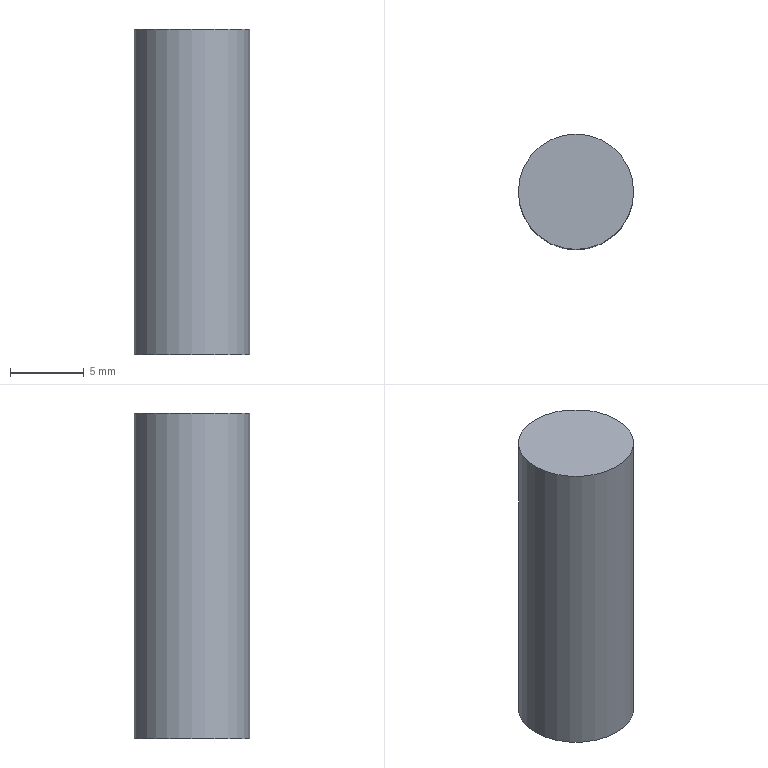Part | NX | features CYLINDER 1, DATUM_CSYS 1 | 1 solid | 3 faces | box 7.8 x 7.8 x 22 mm | volume 1051 mm3 | plane 2 | cylinder 1 | commonest cylinder face diameters 7.8 x1
STEP:
#1=CARTESIAN_POINT('',(3.9,0.,22.));
#2=VERTEX_POINT('',#1);
#3=CARTESIAN_POINT('',(0.,0.,22.));
#4=DIRECTION('',(0.,0.,-1.));
#5=DIRECTION('',(1.,0.,0.));
#6=AXIS2_PLACEMENT_3D('',#3,#4,#5);
#7=CIRCLE('',#6,3.9);
#8=EDGE_CURVE('',#2,#2,#7,.T.);
#9=ORIENTED_EDGE('',*,*,#8,.F.);
#10=EDGE_LOOP('',(#9));
#11=FACE_BOUND('',#10,.T.);
#12=CARTESIAN_POINT('',(0.,0.,22.));
#13=DIRECTION('',(0.,0.,1.));
#14=DIRECTION('',(1.,0.,0.));
#15=AXIS2_PLACEMENT_3D('',#12,#13,#14);
#16=PLANE('',#15);
#17=ADVANCED_FACE('',(#11),#16,.T.);
#18=CARTESIAN_POINT('',(3.9,0.,0.));
#19=VERTEX_POINT('',#18);
#20=CARTESIAN_POINT('',(0.,0.,0.));
#21=DIRECTION('',(0.,0.,1.));
#22=DIRECTION('',(1.,0.,0.));
#23=AXIS2_PLACEMENT_3D('',#20,#21,#22);
#24=CIRCLE('',#23,3.9);
#25=EDGE_CURVE('',#19,#19,#24,.T.);
#26=ORIENTED_EDGE('',*,*,#25,.F.);
#27=EDGE_LOOP('',(#26));
#28=FACE_BOUND('',#27,.T.);
#29=CARTESIAN_POINT('',(0.,0.,0.));
#30=DIRECTION('',(0.,0.,-1.));
#31=DIRECTION('',(-1.,0.,0.));
#32=AXIS2_PLACEMENT_3D('',#29,#30,#31);
#33=PLANE('',#32);
#34=ADVANCED_FACE('',(#28),#33,.T.);
#35=ORIENTED_EDGE('',*,*,#8,.T.);
#36=EDGE_LOOP('',(#35));
#37=FACE_BOUND('',#36,.T.);
#38=ORIENTED_EDGE('',*,*,#25,.T.);
#39=EDGE_LOOP('',(#38));
#40=FACE_BOUND('',#39,.T.);
#41=CARTESIAN_POINT('',(0.,0.,0.));
#42=DIRECTION('',(0.,0.,1.));
#43=DIRECTION('',(1.,0.,0.));
#44=AXIS2_PLACEMENT_3D('',#41,#42,#43);
#45=CYLINDRICAL_SURFACE('',#44,3.9);
#46=ADVANCED_FACE('',(#37,#40),#45,.T.);
#47=CLOSED_SHELL('',(#17,#34,#46));
#48=MANIFOLD_SOLID_BREP('',#47);
#49=(LENGTH_UNIT()NAMED_UNIT(*)SI_UNIT(.MILLI.,.METRE.));
#50=UNCERTAINTY_MEASURE_WITH_UNIT(LENGTH_MEASURE(0.00001),#49,'','');
#51=(NAMED_UNIT(*)PLANE_ANGLE_UNIT()SI_UNIT($,.RADIAN.));
#52=(NAMED_UNIT(*)SI_UNIT($,.STERADIAN.)SOLID_ANGLE_UNIT());
#53=(GEOMETRIC_REPRESENTATION_CONTEXT(3)GLOBAL_UNCERTAINTY_ASSIGNED_CONTEXT((#50))GLOBAL_UNIT_ASSIGNED_CONTEXT((#49,#51,#52))REPRESENTATION_CONTEXT('',''));
#54=ADVANCED_BREP_SHAPE_REPRESENTATION('',(#48),#53);